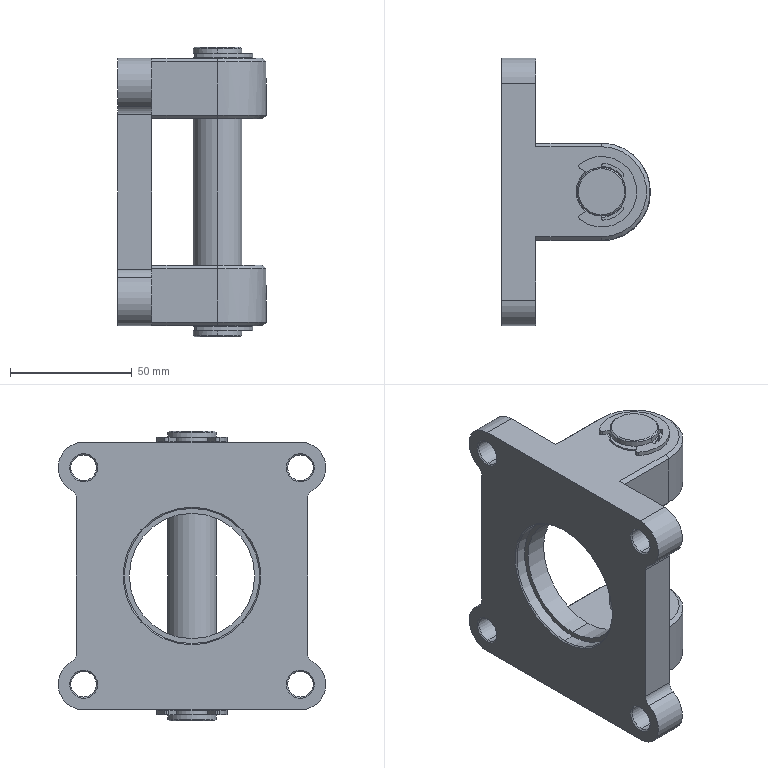Part | STEP file | _F-SE100CB | 1 solid | 164 faces | box 61 x 110 x 119 mm | volume 221745 mm3 | cylinder 69 | plane 55 | cone 40 | commonest cylinder face diameters 1.6 x10 20 x10 10.5 x8 16.5 x8 2.4 x6 15 x6